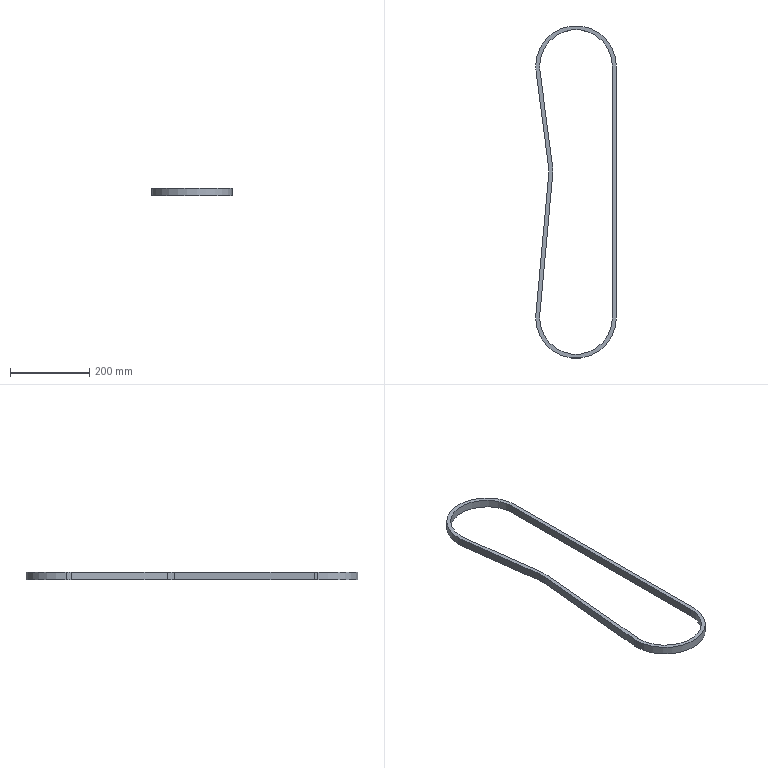Part | SolidWorks | features BeltProfileFeature 1, ExtruThin 1 | 1 solid | 18 faces | box 203.25 x 838.25 x 20 mm | volume 376153 mm3 | cylinder 10 | plane 8 | commonest cylinder face diameters 183.25 x5 203.25 x4 163.25 x1
STEP:
#1=CARTESIAN_POINT('',(-91.239,-626.594,10.));
#2=VERTEX_POINT('',#1);
#3=CARTESIAN_POINT('',(-91.625,-635.,10.));
#4=VERTEX_POINT('',#3);
#5=CARTESIAN_POINT('',(-0.000000034,-635.,10.));
#6=DIRECTION('',(0.,0.,1.));
#7=DIRECTION('',(-1.,0.,0.));
#8=AXIS2_PLACEMENT_3D('',#5,#6,#7);
#9=CIRCLE('',#8,91.625);
#10=EDGE_CURVE('',#2,#4,#9,.T.);
#11=ORIENTED_EDGE('',*,*,#10,.T.);
#12=CARTESIAN_POINT('',(-91.625,-635.,-10.));
#13=VERTEX_POINT('',#12);
#14=CARTESIAN_POINT('',(-91.625,-635.,10.));
#15=DIRECTION('',(0.,0.,-1.));
#16=VECTOR('',#15,1000.);
#17=LINE('',#14,#16);
#18=EDGE_CURVE('',#4,#13,#17,.T.);
#19=ORIENTED_EDGE('',*,*,#18,.T.);
#20=CARTESIAN_POINT('',(-91.239,-626.594,-10.));
#21=VERTEX_POINT('',#20);
#22=CARTESIAN_POINT('',(-0.000000034,-635.,-10.));
#23=DIRECTION('',(0.,0.,1.));
#24=DIRECTION('',(-1.,0.,0.));
#25=AXIS2_PLACEMENT_3D('',#22,#23,#24);
#26=CIRCLE('',#25,91.625);
#27=EDGE_CURVE('',#21,#13,#26,.T.);
#28=ORIENTED_EDGE('',*,*,#27,.F.);
#29=CARTESIAN_POINT('',(-91.239,-626.594,10.));
#30=DIRECTION('',(0.,0.,-1.));
#31=VECTOR('',#30,1000.);
#32=LINE('',#29,#31);
#33=EDGE_CURVE('',#2,#21,#32,.T.);
#34=ORIENTED_EDGE('',*,*,#33,.F.);
#35=EDGE_LOOP('',(#11,#19,#28,#34));
#36=FACE_OUTER_BOUND('',#35,.T.);
#37=CARTESIAN_POINT('',(-0.000000034,-635.,10.));
#38=DIRECTION('',(0.,0.,-1.));
#39=DIRECTION('',(-1.,0.,0.));
#40=AXIS2_PLACEMENT_3D('',#37,#38,#39);
#41=CYLINDRICAL_SURFACE('',#40,91.625);
#42=ADVANCED_FACE('',(#36),#41,.F.);
#43=CARTESIAN_POINT('',(91.625,0.000000022,10.));
#44=VERTEX_POINT('',#43);
#45=CARTESIAN_POINT('',(-91.625,0.000000021,10.));
#46=VERTEX_POINT('',#45);
#47=CARTESIAN_POINT('',(-0.000000034,0.000000021,10.));
#48=DIRECTION('',(0.,0.,1.));
#49=DIRECTION('',(-1.,0.,0.));
#50=AXIS2_PLACEMENT_3D('',#47,#48,#49);
#51=CIRCLE('',#50,91.625);
#52=EDGE_CURVE('',#44,#46,#51,.T.);
#53=ORIENTED_EDGE('',*,*,#52,.T.);
#54=CARTESIAN_POINT('',(-91.625,0.000000021,-10.));
#55=VERTEX_POINT('',#54);
#56=CARTESIAN_POINT('',(-91.625,0.000000021,10.));
#57=DIRECTION('',(0.,0.,-1.));
#58=VECTOR('',#57,1000.);
#59=LINE('',#56,#58);
#60=EDGE_CURVE('',#46,#55,#59,.T.);
#61=ORIENTED_EDGE('',*,*,#60,.T.);
#62=CARTESIAN_POINT('',(91.625,0.000000022,-10.));
#63=VERTEX_POINT('',#62);
#64=CARTESIAN_POINT('',(-0.000000034,0.000000021,-10.));
#65=DIRECTION('',(0.,0.,1.));
#66=DIRECTION('',(-1.,0.,0.));
#67=AXIS2_PLACEMENT_3D('',#64,#65,#66);
#68=CIRCLE('',#67,91.625);
#69=EDGE_CURVE('',#63,#55,#68,.T.);
#70=ORIENTED_EDGE('',*,*,#69,.F.);
#71=CARTESIAN_POINT('',(91.625,0.000000022,10.));
#72=DIRECTION('',(0.,0.,-1.));
#73=VECTOR('',#72,1000.);
#74=LINE('',#71,#73);
#75=EDGE_CURVE('',#44,#63,#74,.T.);
#76=ORIENTED_EDGE('',*,*,#75,.F.);
#77=EDGE_LOOP('',(#53,#61,#70,#76));
#78=FACE_OUTER_BOUND('',#77,.T.);
#79=CARTESIAN_POINT('',(-0.000000034,0.000000021,10.));
#80=DIRECTION('',(0.,0.,-1.));
#81=DIRECTION('',(-1.,0.,0.));
#82=AXIS2_PLACEMENT_3D('',#79,#80,#81);
#83=CYLINDRICAL_SURFACE('',#82,91.625);
#84=ADVANCED_FACE('',(#78),#83,.F.);
#85=CARTESIAN_POINT('',(-101.625,-635.,10.));
#86=VERTEX_POINT('',#85);
#87=CARTESIAN_POINT('',(101.625,-635.,10.));
#88=VERTEX_POINT('',#87);
#89=CARTESIAN_POINT('',(-0.000000034,-635.,10.));
#90=DIRECTION('',(0.,0.,1.));
#91=DIRECTION('',(-1.,0.,0.));
#92=AXIS2_PLACEMENT_3D('',#89,#90,#91);
#93=CIRCLE('',#92,101.625);
#94=EDGE_CURVE('',#86,#88,#93,.T.);
#95=ORIENTED_EDGE('',*,*,#94,.F.);
#96=CARTESIAN_POINT('',(-101.625,-635.,-10.));
#97=VERTEX_POINT('',#96);
#98=CARTESIAN_POINT('',(-101.625,-635.,10.));
#99=DIRECTION('',(0.,0.,-1.));
#100=VECTOR('',#99,1000.);
#101=LINE('',#98,#100);
#102=EDGE_CURVE('',#86,#97,#101,.T.);
#103=ORIENTED_EDGE('',*,*,#102,.T.);
#104=CARTESIAN_POINT('',(101.625,-635.,-10.));
#105=VERTEX_POINT('',#104);
#106=CARTESIAN_POINT('',(-0.000000034,-635.,-10.));
#107=DIRECTION('',(0.,0.,1.));
#108=DIRECTION('',(-1.,0.,0.));
#109=AXIS2_PLACEMENT_3D('',#106,#107,#108);
#110=CIRCLE('',#109,101.625);
#111=EDGE_CURVE('',#97,#105,#110,.T.);
#112=ORIENTED_EDGE('',*,*,#111,.T.);
#113=CARTESIAN_POINT('',(101.625,-635.,10.));
#114=DIRECTION('',(0.,0.,-1.));
#115=VECTOR('',#114,1000.);
#116=LINE('',#113,#115);
#117=EDGE_CURVE('',#88,#105,#116,.T.);
#118=ORIENTED_EDGE('',*,*,#117,.F.);
#119=EDGE_LOOP('',(#95,#103,#112,#118));
#120=FACE_OUTER_BOUND('',#119,.T.);
#121=CARTESIAN_POINT('',(-0.000000034,-635.,10.));
#122=DIRECTION('',(0.,0.,-1.));
#123=DIRECTION('',(-1.,0.,0.));
#124=AXIS2_PLACEMENT_3D('',#121,#122,#123);
#125=CYLINDRICAL_SURFACE('',#124,101.625);
#126=ADVANCED_FACE('',(#120),#125,.T.);
#127=CARTESIAN_POINT('',(-101.625,0.000000021,10.));
#128=VERTEX_POINT('',#127);
#129=CARTESIAN_POINT('',(-100.763,-13.206,10.));
#130=VERTEX_POINT('',#129);
#131=CARTESIAN_POINT('',(-0.000000034,0.000000021,10.));
#132=DIRECTION('',(0.,0.,1.));
#133=DIRECTION('',(-1.,0.,0.));
#134=AXIS2_PLACEMENT_3D('',#131,#132,#133);
#135=CIRCLE('',#134,101.625);
#136=EDGE_CURVE('',#128,#130,#135,.T.);
#137=ORIENTED_EDGE('',*,*,#136,.F.);
#138=CARTESIAN_POINT('',(-101.625,0.000000021,-10.));
#139=VERTEX_POINT('',#138);
#140=CARTESIAN_POINT('',(-101.625,0.000000021,10.));
#141=DIRECTION('',(0.,0.,-1.));
#142=VECTOR('',#141,1000.);
#143=LINE('',#140,#142);
#144=EDGE_CURVE('',#128,#139,#143,.T.);
#145=ORIENTED_EDGE('',*,*,#144,.T.);
#146=CARTESIAN_POINT('',(-100.763,-13.206,-10.));
#147=VERTEX_POINT('',#146);
#148=CARTESIAN_POINT('',(-0.000000034,0.000000021,-10.));
#149=DIRECTION('',(0.,0.,1.));
#150=DIRECTION('',(-1.,0.,0.));
#151=AXIS2_PLACEMENT_3D('',#148,#149,#150);
#152=CIRCLE('',#151,101.625);
#153=EDGE_CURVE('',#139,#147,#152,.T.);
#154=ORIENTED_EDGE('',*,*,#153,.T.);
#155=CARTESIAN_POINT('',(-100.763,-13.206,10.));
#156=DIRECTION('',(0.,0.,-1.));
#157=VECTOR('',#156,1000.);
#158=LINE('',#155,#157);
#159=EDGE_CURVE('',#130,#147,#158,.T.);
#160=ORIENTED_EDGE('',*,*,#159,.F.);
#161=EDGE_LOOP('',(#137,#145,#154,#160));
#162=FACE_OUTER_BOUND('',#161,.T.);
#163=CARTESIAN_POINT('',(-0.000000034,0.000000021,10.));
#164=DIRECTION('',(0.,0.,-1.));
#165=DIRECTION('',(-1.,0.,0.));
#166=AXIS2_PLACEMENT_3D('',#163,#164,#165);
#167=CYLINDRICAL_SURFACE('',#166,101.625);
#168=ADVANCED_FACE('',(#162),#167,.T.);
#169=CARTESIAN_POINT('',(101.625,0.000000022,10.));
#170=VERTEX_POINT('',#169);
#171=CARTESIAN_POINT('',(-0.000000034,0.000000021,10.));
#172=DIRECTION('',(0.,0.,1.));
#173=DIRECTION('',(-1.,0.,0.));
#174=AXIS2_PLACEMENT_3D('',#171,#172,#173);
#175=CIRCLE('',#174,101.625);
#176=EDGE_CURVE('',#170,#128,#175,.T.);
#177=ORIENTED_EDGE('',*,*,#176,.T.);
#178=ORIENTED_EDGE('',*,*,#136,.T.);
#179=CARTESIAN_POINT('',(-69.067,-255.055,10.));
#180=VERTEX_POINT('',#179);
#181=CARTESIAN_POINT('',(-100.763,-13.206,10.));
#182=DIRECTION('',(0.1299,-0.9915,0.));
#183=VECTOR('',#182,1000.);
#184=LINE('',#181,#183);
#185=EDGE_CURVE('',#130,#180,#184,.T.);
#186=ORIENTED_EDGE('',*,*,#185,.T.);
#187=CARTESIAN_POINT('',(-68.719,-273.15,10.));
#188=VERTEX_POINT('',#187);
#189=CARTESIAN_POINT('',(-150.,-265.662,10.));
#190=DIRECTION('',(0.,0.,-1.));
#191=DIRECTION('',(-1.,0.,0.));
#192=AXIS2_PLACEMENT_3D('',#189,#190,#191);
#193=CIRCLE('',#192,81.625);
#194=EDGE_CURVE('',#180,#188,#193,.T.);
#195=ORIENTED_EDGE('',*,*,#194,.T.);
#196=CARTESIAN_POINT('',(-101.196,-625.677,10.));
#197=VERTEX_POINT('',#196);
#198=CARTESIAN_POINT('',(-43.188,3.979,10.));
#199=DIRECTION('',(-0.09174,-0.9958,0.));
#200=VECTOR('',#199,1000.);
#201=LINE('',#198,#200);
#202=EDGE_CURVE('',#188,#197,#201,.T.);
#203=ORIENTED_EDGE('',*,*,#202,.T.);
#204=CARTESIAN_POINT('',(-0.000000034,-635.,10.));
#205=DIRECTION('',(0.,0.,1.));
#206=DIRECTION('',(-1.,0.,0.));
#207=AXIS2_PLACEMENT_3D('',#204,#205,#206);
#208=CIRCLE('',#207,101.625);
#209=EDGE_CURVE('',#197,#86,#208,.T.);
#210=ORIENTED_EDGE('',*,*,#209,.T.);
#211=ORIENTED_EDGE('',*,*,#94,.T.);
#212=CARTESIAN_POINT('',(101.625,0.000000021,10.));
#213=DIRECTION('',(0.,1.,0.));
#214=VECTOR('',#213,1000.);
#215=LINE('',#212,#214);
#216=EDGE_CURVE('',#88,#170,#215,.T.);
#217=ORIENTED_EDGE('',*,*,#216,.T.);
#218=EDGE_LOOP('',(#177,#178,#186,#195,#203,#210,#211,#217));
#219=FACE_OUTER_BOUND('',#218,.T.);
#220=ORIENTED_EDGE('',*,*,#52,.F.);
#221=CARTESIAN_POINT('',(91.625,-635.,10.));
#222=VERTEX_POINT('',#221);
#223=CARTESIAN_POINT('',(91.625,0.000000022,10.));
#224=DIRECTION('',(0.,1.,0.));
#225=VECTOR('',#224,1000.);
#226=LINE('',#223,#225);
#227=EDGE_CURVE('',#222,#44,#226,.T.);
#228=ORIENTED_EDGE('',*,*,#227,.F.);
#229=CARTESIAN_POINT('',(-0.000000034,-635.,10.));
#230=DIRECTION('',(0.,0.,1.));
#231=DIRECTION('',(-1.,0.,0.));
#232=AXIS2_PLACEMENT_3D('',#229,#230,#231);
#233=CIRCLE('',#232,91.625);
#234=EDGE_CURVE('',#4,#222,#233,.T.);
#235=ORIENTED_EDGE('',*,*,#234,.F.);
#236=ORIENTED_EDGE('',*,*,#10,.F.);
#237=CARTESIAN_POINT('',(-58.761,-274.068,10.));
#238=VERTEX_POINT('',#237);
#239=CARTESIAN_POINT('',(-91.239,-626.594,10.));
#240=DIRECTION('',(-0.09174,-0.9958,0.));
#241=VECTOR('',#240,1000.);
#242=LINE('',#239,#241);
#243=EDGE_CURVE('',#238,#2,#242,.T.);
#244=ORIENTED_EDGE('',*,*,#243,.F.);
#245=CARTESIAN_POINT('',(-59.152,-253.756,10.));
#246=VERTEX_POINT('',#245);
#247=CARTESIAN_POINT('',(-150.,-265.662,10.));
#248=DIRECTION('',(0.,0.,-1.));
#249=DIRECTION('',(1.,0.,0.));
#250=AXIS2_PLACEMENT_3D('',#247,#248,#249);
#251=CIRCLE('',#250,91.625);
#252=EDGE_CURVE('',#246,#238,#251,.T.);
#253=ORIENTED_EDGE('',*,*,#252,.F.);
#254=CARTESIAN_POINT('',(-90.848,-11.906,10.));
#255=VERTEX_POINT('',#254);
#256=CARTESIAN_POINT('',(-59.152,-253.756,10.));
#257=DIRECTION('',(0.1299,-0.9915,0.));
#258=VECTOR('',#257,1000.);
#259=LINE('',#256,#258);
#260=EDGE_CURVE('',#255,#246,#259,.T.);
#261=ORIENTED_EDGE('',*,*,#260,.F.);
#262=CARTESIAN_POINT('',(-0.000000034,0.000000021,10.));
#263=DIRECTION('',(0.,0.,1.));
#264=DIRECTION('',(-1.,0.,0.));
#265=AXIS2_PLACEMENT_3D('',#262,#263,#264);
#266=CIRCLE('',#265,91.625);
#267=EDGE_CURVE('',#46,#255,#266,.T.);
#268=ORIENTED_EDGE('',*,*,#267,.F.);
#269=EDGE_LOOP('',(#220,#228,#235,#236,#244,#253,#261,#268));
#270=FACE_BOUND('',#269,.T.);
#271=CARTESIAN_POINT('',(-0.000000034,0.000000021,10.));
#272=DIRECTION('',(0.,0.,-1.));
#273=DIRECTION('',(-1.,0.,0.));
#274=AXIS2_PLACEMENT_3D('',#271,#272,#273);
#275=PLANE('',#274);
#276=ADVANCED_FACE('',(#219,#270),#275,.F.);
#277=CARTESIAN_POINT('',(101.625,0.000000022,-10.));
#278=VERTEX_POINT('',#277);
#279=CARTESIAN_POINT('',(-0.000000034,0.000000021,-10.));
#280=DIRECTION('',(0.,0.,1.));
#281=DIRECTION('',(-1.,0.,0.));
#282=AXIS2_PLACEMENT_3D('',#279,#280,#281);
#283=CIRCLE('',#282,101.625);
#284=EDGE_CURVE('',#278,#139,#283,.T.);
#285=ORIENTED_EDGE('',*,*,#284,.F.);
#286=CARTESIAN_POINT('',(101.625,0.000000021,-10.));
#287=DIRECTION('',(0.,1.,0.));
#288=VECTOR('',#287,1000.);
#289=LINE('',#286,#288);
#290=EDGE_CURVE('',#105,#278,#289,.T.);
#291=ORIENTED_EDGE('',*,*,#290,.F.);
#292=ORIENTED_EDGE('',*,*,#111,.F.);
#293=CARTESIAN_POINT('',(-101.196,-625.677,-10.));
#294=VERTEX_POINT('',#293);
#295=CARTESIAN_POINT('',(-0.000000034,-635.,-10.));
#296=DIRECTION('',(0.,0.,1.));
#297=DIRECTION('',(-1.,0.,0.));
#298=AXIS2_PLACEMENT_3D('',#295,#296,#297);
#299=CIRCLE('',#298,101.625);
#300=EDGE_CURVE('',#294,#97,#299,.T.);
#301=ORIENTED_EDGE('',*,*,#300,.F.);
#302=CARTESIAN_POINT('',(-68.719,-273.15,-10.));
#303=VERTEX_POINT('',#302);
#304=CARTESIAN_POINT('',(-43.188,3.979,-10.));
#305=DIRECTION('',(-0.09174,-0.9958,0.));
#306=VECTOR('',#305,1000.);
#307=LINE('',#304,#306);
#308=EDGE_CURVE('',#303,#294,#307,.T.);
#309=ORIENTED_EDGE('',*,*,#308,.F.);
#310=CARTESIAN_POINT('',(-69.067,-255.055,-10.));
#311=VERTEX_POINT('',#310);
#312=CARTESIAN_POINT('',(-150.,-265.662,-10.));
#313=DIRECTION('',(0.,0.,-1.));
#314=DIRECTION('',(-1.,0.,0.));
#315=AXIS2_PLACEMENT_3D('',#312,#313,#314);
#316=CIRCLE('',#315,81.625);
#317=EDGE_CURVE('',#311,#303,#316,.T.);
#318=ORIENTED_EDGE('',*,*,#317,.F.);
#319=CARTESIAN_POINT('',(-100.763,-13.206,-10.));
#320=DIRECTION('',(0.1299,-0.9915,0.));
#321=VECTOR('',#320,1000.);
#322=LINE('',#319,#321);
#323=EDGE_CURVE('',#147,#311,#322,.T.);
#324=ORIENTED_EDGE('',*,*,#323,.F.);
#325=ORIENTED_EDGE('',*,*,#153,.F.);
#326=EDGE_LOOP('',(#285,#291,#292,#301,#309,#318,#324,#325));
#327=FACE_OUTER_BOUND('',#326,.T.);
#328=CARTESIAN_POINT('',(91.625,-635.,-10.));
#329=VERTEX_POINT('',#328);
#330=CARTESIAN_POINT('',(91.625,0.000000022,-10.));
#331=DIRECTION('',(0.,1.,0.));
#332=VECTOR('',#331,1000.);
#333=LINE('',#330,#332);
#334=EDGE_CURVE('',#329,#63,#333,.T.);
#335=ORIENTED_EDGE('',*,*,#334,.T.);
#336=ORIENTED_EDGE('',*,*,#69,.T.);
#337=CARTESIAN_POINT('',(-90.848,-11.906,-10.));
#338=VERTEX_POINT('',#337);
#339=CARTESIAN_POINT('',(-0.000000034,0.000000021,-10.));
#340=DIRECTION('',(0.,0.,1.));
#341=DIRECTION('',(-1.,0.,0.));
#342=AXIS2_PLACEMENT_3D('',#339,#340,#341);
#343=CIRCLE('',#342,91.625);
#344=EDGE_CURVE('',#55,#338,#343,.T.);
#345=ORIENTED_EDGE('',*,*,#344,.T.);
#346=CARTESIAN_POINT('',(-59.152,-253.756,-10.));
#347=VERTEX_POINT('',#346);
#348=CARTESIAN_POINT('',(-59.152,-253.756,-10.));
#349=DIRECTION('',(0.1299,-0.9915,0.));
#350=VECTOR('',#349,1000.);
#351=LINE('',#348,#350);
#352=EDGE_CURVE('',#338,#347,#351,.T.);
#353=ORIENTED_EDGE('',*,*,#352,.T.);
#354=CARTESIAN_POINT('',(-58.761,-274.068,-10.));
#355=VERTEX_POINT('',#354);
#356=CARTESIAN_POINT('',(-150.,-265.662,-10.));
#357=DIRECTION('',(0.,0.,-1.));
#358=DIRECTION('',(1.,0.,0.));
#359=AXIS2_PLACEMENT_3D('',#356,#357,#358);
#360=CIRCLE('',#359,91.625);
#361=EDGE_CURVE('',#347,#355,#360,.T.);
#362=ORIENTED_EDGE('',*,*,#361,.T.);
#363=CARTESIAN_POINT('',(-91.239,-626.594,-10.));
#364=DIRECTION('',(-0.09174,-0.9958,0.));
#365=VECTOR('',#364,1000.);
#366=LINE('',#363,#365);
#367=EDGE_CURVE('',#355,#21,#366,.T.);
#368=ORIENTED_EDGE('',*,*,#367,.T.);
#369=ORIENTED_EDGE('',*,*,#27,.T.);
#370=CARTESIAN_POINT('',(-0.000000034,-635.,-10.));
#371=DIRECTION('',(0.,0.,1.));
#372=DIRECTION('',(-1.,0.,0.));
#373=AXIS2_PLACEMENT_3D('',#370,#371,#372);
#374=CIRCLE('',#373,91.625);
#375=EDGE_CURVE('',#13,#329,#374,.T.);
#376=ORIENTED_EDGE('',*,*,#375,.T.);
#377=EDGE_LOOP('',(#335,#336,#345,#353,#362,#368,#369,#376));
#378=FACE_BOUND('',#377,.T.);
#379=CARTESIAN_POINT('',(-0.000000034,0.000000021,-10.));
#380=DIRECTION('',(0.,0.,-1.));
#381=DIRECTION('',(-1.,0.,0.));
#382=AXIS2_PLACEMENT_3D('',#379,#380,#381);
#383=PLANE('',#382);
#384=ADVANCED_FACE('',(#327,#378),#383,.T.);
#385=ORIENTED_EDGE('',*,*,#144,.F.);
#386=ORIENTED_EDGE('',*,*,#176,.F.);
#387=CARTESIAN_POINT('',(101.625,0.000000022,10.));
#388=DIRECTION('',(0.,0.,-1.));
#389=VECTOR('',#388,1000.);
#390=LINE('',#387,#389);
#391=EDGE_CURVE('',#170,#278,#390,.T.);
#392=ORIENTED_EDGE('',*,*,#391,.T.);
#393=ORIENTED_EDGE('',*,*,#284,.T.);
#394=EDGE_LOOP('',(#385,#386,#392,#393));
#395=FACE_OUTER_BOUND('',#394,.T.);
#396=CARTESIAN_POINT('',(-0.000000034,0.000000021,10.));
#397=DIRECTION('',(0.,0.,-1.));
#398=DIRECTION('',(-1.,0.,0.));
#399=AXIS2_PLACEMENT_3D('',#396,#397,#398);
#400=CYLINDRICAL_SURFACE('',#399,101.625);
#401=ADVANCED_FACE('',(#395),#400,.T.);
#402=ORIENTED_EDGE('',*,*,#323,.T.);
#403=CARTESIAN_POINT('',(-69.067,-255.055,10.));
#404=DIRECTION('',(0.,0.,-1.));
#405=VECTOR('',#404,1000.);
#406=LINE('',#403,#405);
#407=EDGE_CURVE('',#180,#311,#406,.T.);
#408=ORIENTED_EDGE('',*,*,#407,.F.);
#409=ORIENTED_EDGE('',*,*,#185,.F.);
#410=ORIENTED_EDGE('',*,*,#159,.T.);
#411=EDGE_LOOP('',(#402,#408,#409,#410));
#412=FACE_OUTER_BOUND('',#411,.T.);
#413=CARTESIAN_POINT('',(-100.763,-13.206,10.));
#414=DIRECTION('',(0.9915,0.1299,0.));
#415=DIRECTION('',(-0.1299,0.9915,0.));
#416=AXIS2_PLACEMENT_3D('',#413,#414,#415);
#417=PLANE('',#416);
#418=ADVANCED_FACE('',(#412),#417,.F.);
#419=ORIENTED_EDGE('',*,*,#317,.T.);
#420=CARTESIAN_POINT('',(-68.719,-273.15,10.));
#421=DIRECTION('',(0.,0.,-1.));
#422=VECTOR('',#421,1000.);
#423=LINE('',#420,#422);
#424=EDGE_CURVE('',#188,#303,#423,.T.);
#425=ORIENTED_EDGE('',*,*,#424,.F.);
#426=ORIENTED_EDGE('',*,*,#194,.F.);
#427=ORIENTED_EDGE('',*,*,#407,.T.);
#428=EDGE_LOOP('',(#419,#425,#426,#427));
#429=FACE_OUTER_BOUND('',#428,.T.);
#430=CARTESIAN_POINT('',(-150.,-265.662,10.));
#431=DIRECTION('',(0.,0.,-1.));
#432=DIRECTION('',(-1.,0.,0.));
#433=AXIS2_PLACEMENT_3D('',#430,#431,#432);
#434=CYLINDRICAL_SURFACE('',#433,81.625);
#435=ADVANCED_FACE('',(#429),#434,.F.);
#436=ORIENTED_EDGE('',*,*,#308,.T.);
#437=CARTESIAN_POINT('',(-101.196,-625.677,10.));
#438=DIRECTION('',(0.,0.,-1.));
#439=VECTOR('',#438,1000.);
#440=LINE('',#437,#439);
#441=EDGE_CURVE('',#197,#294,#440,.T.);
#442=ORIENTED_EDGE('',*,*,#441,.F.);
#443=ORIENTED_EDGE('',*,*,#202,.F.);
#444=ORIENTED_EDGE('',*,*,#424,.T.);
#445=EDGE_LOOP('',(#436,#442,#443,#444));
#446=FACE_OUTER_BOUND('',#445,.T.);
#447=CARTESIAN_POINT('',(-43.188,3.979,10.));
#448=DIRECTION('',(0.9958,-0.09174,0.));
#449=DIRECTION('',(0.09174,0.9958,0.));
#450=AXIS2_PLACEMENT_3D('',#447,#448,#449);
#451=PLANE('',#450);
#452=ADVANCED_FACE('',(#446),#451,.F.);
#453=ORIENTED_EDGE('',*,*,#102,.F.);
#454=ORIENTED_EDGE('',*,*,#209,.F.);
#455=ORIENTED_EDGE('',*,*,#441,.T.);
#456=ORIENTED_EDGE('',*,*,#300,.T.);
#457=EDGE_LOOP('',(#453,#454,#455,#456));
#458=FACE_OUTER_BOUND('',#457,.T.);
#459=CARTESIAN_POINT('',(-0.000000034,-635.,10.));
#460=DIRECTION('',(0.,0.,-1.));
#461=DIRECTION('',(-1.,0.,0.));
#462=AXIS2_PLACEMENT_3D('',#459,#460,#461);
#463=CYLINDRICAL_SURFACE('',#462,101.625);
#464=ADVANCED_FACE('',(#458),#463,.T.);
#465=ORIENTED_EDGE('',*,*,#290,.T.);
#466=ORIENTED_EDGE('',*,*,#391,.F.);
#467=ORIENTED_EDGE('',*,*,#216,.F.);
#468=ORIENTED_EDGE('',*,*,#117,.T.);
#469=EDGE_LOOP('',(#465,#466,#467,#468));
#470=FACE_OUTER_BOUND('',#469,.T.);
#471=CARTESIAN_POINT('',(101.625,0.000000021,10.));
#472=DIRECTION('',(-1.,0.,0.));
#473=DIRECTION('',(0.,0.,1.));
#474=AXIS2_PLACEMENT_3D('',#471,#472,#473);
#475=PLANE('',#474);
#476=ADVANCED_FACE('',(#470),#475,.F.);
#477=ORIENTED_EDGE('',*,*,#60,.F.);
#478=ORIENTED_EDGE('',*,*,#267,.T.);
#479=CARTESIAN_POINT('',(-90.848,-11.906,10.));
#480=DIRECTION('',(0.,0.,-1.));
#481=VECTOR('',#480,1000.);
#482=LINE('',#479,#481);
#483=EDGE_CURVE('',#255,#338,#482,.T.);
#484=ORIENTED_EDGE('',*,*,#483,.T.);
#485=ORIENTED_EDGE('',*,*,#344,.F.);
#486=EDGE_LOOP('',(#477,#478,#484,#485));
#487=FACE_OUTER_BOUND('',#486,.T.);
#488=CARTESIAN_POINT('',(-0.000000034,0.000000021,10.));
#489=DIRECTION('',(0.,0.,-1.));
#490=DIRECTION('',(-1.,0.,0.));
#491=AXIS2_PLACEMENT_3D('',#488,#489,#490);
#492=CYLINDRICAL_SURFACE('',#491,91.625);
#493=ADVANCED_FACE('',(#487),#492,.F.);
#494=ORIENTED_EDGE('',*,*,#352,.F.);
#495=ORIENTED_EDGE('',*,*,#483,.F.);
#496=ORIENTED_EDGE('',*,*,#260,.T.);
#497=CARTESIAN_POINT('',(-59.152,-253.756,10.));
#498=DIRECTION('',(0.,0.,-1.));
#499=VECTOR('',#498,1000.);
#500=LINE('',#497,#499);
#501=EDGE_CURVE('',#246,#347,#500,.T.);
#502=ORIENTED_EDGE('',*,*,#501,.T.);
#503=EDGE_LOOP('',(#494,#495,#496,#502));
#504=FACE_OUTER_BOUND('',#503,.T.);
#505=CARTESIAN_POINT('',(-59.152,-253.756,10.));
#506=DIRECTION('',(0.9915,0.1299,0.));
#507=DIRECTION('',(-0.1299,0.9915,0.));
#508=AXIS2_PLACEMENT_3D('',#505,#506,#507);
#509=PLANE('',#508);
#510=ADVANCED_FACE('',(#504),#509,.T.);
#511=ORIENTED_EDGE('',*,*,#361,.F.);
#512=ORIENTED_EDGE('',*,*,#501,.F.);
#513=ORIENTED_EDGE('',*,*,#252,.T.);
#514=CARTESIAN_POINT('',(-58.761,-274.068,10.));
#515=DIRECTION('',(0.,0.,-1.));
#516=VECTOR('',#515,1000.);
#517=LINE('',#514,#516);
#518=EDGE_CURVE('',#238,#355,#517,.T.);
#519=ORIENTED_EDGE('',*,*,#518,.T.);
#520=EDGE_LOOP('',(#511,#512,#513,#519));
#521=FACE_OUTER_BOUND('',#520,.T.);
#522=CARTESIAN_POINT('',(-150.,-265.662,10.));
#523=DIRECTION('',(0.,0.,-1.));
#524=DIRECTION('',(-1.,0.,0.));
#525=AXIS2_PLACEMENT_3D('',#522,#523,#524);
#526=CYLINDRICAL_SURFACE('',#525,91.625);
#527=ADVANCED_FACE('',(#521),#526,.T.);
#528=ORIENTED_EDGE('',*,*,#367,.F.);
#529=ORIENTED_EDGE('',*,*,#518,.F.);
#530=ORIENTED_EDGE('',*,*,#243,.T.);
#531=ORIENTED_EDGE('',*,*,#33,.T.);
#532=EDGE_LOOP('',(#528,#529,#530,#531));
#533=FACE_OUTER_BOUND('',#532,.T.);
#534=CARTESIAN_POINT('',(-91.239,-626.594,10.));
#535=DIRECTION('',(0.9958,-0.09174,0.));
#536=DIRECTION('',(0.09174,0.9958,0.));
#537=AXIS2_PLACEMENT_3D('',#534,#535,#536);
#538=PLANE('',#537);
#539=ADVANCED_FACE('',(#533),#538,.T.);
#540=ORIENTED_EDGE('',*,*,#18,.F.);
#541=ORIENTED_EDGE('',*,*,#234,.T.);
#542=CARTESIAN_POINT('',(91.625,-635.,10.));
#543=DIRECTION('',(0.,0.,-1.));
#544=VECTOR('',#543,1000.);
#545=LINE('',#542,#544);
#546=EDGE_CURVE('',#222,#329,#545,.T.);
#547=ORIENTED_EDGE('',*,*,#546,.T.);
#548=ORIENTED_EDGE('',*,*,#375,.F.);
#549=EDGE_LOOP('',(#540,#541,#547,#548));
#550=FACE_OUTER_BOUND('',#549,.T.);
#551=CARTESIAN_POINT('',(-0.000000034,-635.,10.));
#552=DIRECTION('',(0.,0.,-1.));
#553=DIRECTION('',(-1.,0.,0.));
#554=AXIS2_PLACEMENT_3D('',#551,#552,#553);
#555=CYLINDRICAL_SURFACE('',#554,91.625);
#556=ADVANCED_FACE('',(#550),#555,.F.);
#557=ORIENTED_EDGE('',*,*,#334,.F.);
#558=ORIENTED_EDGE('',*,*,#546,.F.);
#559=ORIENTED_EDGE('',*,*,#227,.T.);
#560=ORIENTED_EDGE('',*,*,#75,.T.);
#561=EDGE_LOOP('',(#557,#558,#559,#560));
#562=FACE_OUTER_BOUND('',#561,.T.);
#563=CARTESIAN_POINT('',(91.625,0.000000022,10.));
#564=DIRECTION('',(-1.,0.,0.));
#565=DIRECTION('',(0.,0.,1.));
#566=AXIS2_PLACEMENT_3D('',#563,#564,#565);
#567=PLANE('',#566);
#568=ADVANCED_FACE('',(#562),#567,.T.);
#569=CLOSED_SHELL('',(#42,#84,#126,#168,#276,#384,#401,#418,#435,#452,#464,#476,#493,#510,#527,#539,#556,#568));
#570=MANIFOLD_SOLID_BREP('',#569);
#571=CARTESIAN_POINT('',(0.,0.,0.));
#572=DIRECTION('',(0.,0.,1.));
#573=DIRECTION('',(1.,0.,0.));
#574=AXIS2_PLACEMENT_3D('',#571,#572,#573);
#575=(LENGTH_UNIT()NAMED_UNIT(*)SI_UNIT(.MILLI.,.METRE.));
#576=UNCERTAINTY_MEASURE_WITH_UNIT(LENGTH_MEASURE(0.00001),#575,'','');
#577=(NAMED_UNIT(*)PLANE_ANGLE_UNIT()SI_UNIT($,.RADIAN.));
#578=(NAMED_UNIT(*)SI_UNIT($,.STERADIAN.)SOLID_ANGLE_UNIT());
#579=(GEOMETRIC_REPRESENTATION_CONTEXT(3)GLOBAL_UNCERTAINTY_ASSIGNED_CONTEXT((#576))GLOBAL_UNIT_ASSIGNED_CONTEXT((#575,#577,#578))REPRESENTATION_CONTEXT('',''));
#580=ADVANCED_BREP_SHAPE_REPRESENTATION('',(#570,#574),#579);